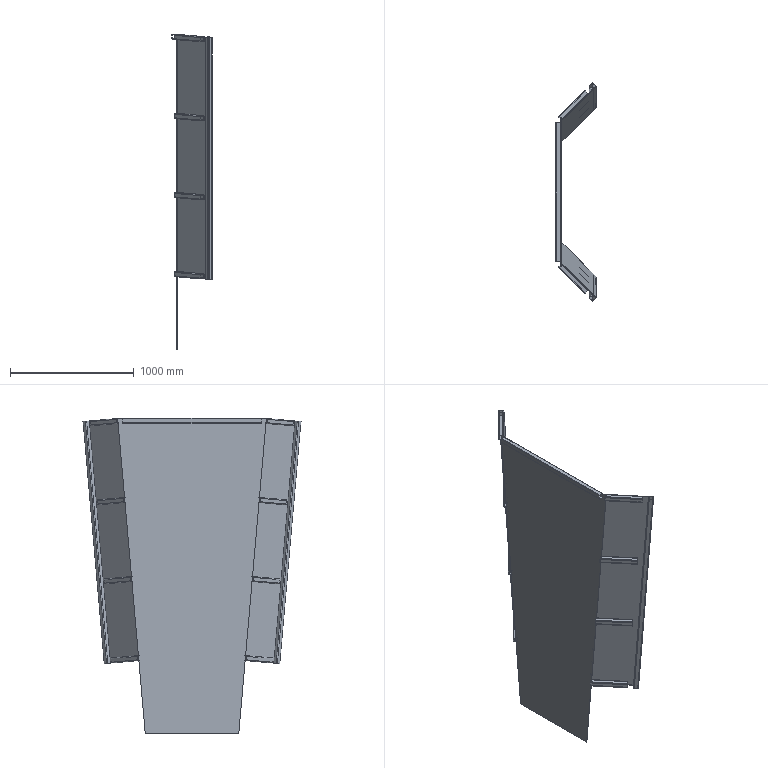Part | STEP file | COMPOUND | 14 solids | 216 faces | box 325.47 x 1761 x 2548 mm | volume 11145517 mm3 | plane 128 | cylinder 88 | commonest cylinder face diameters 6 x44 12 x44